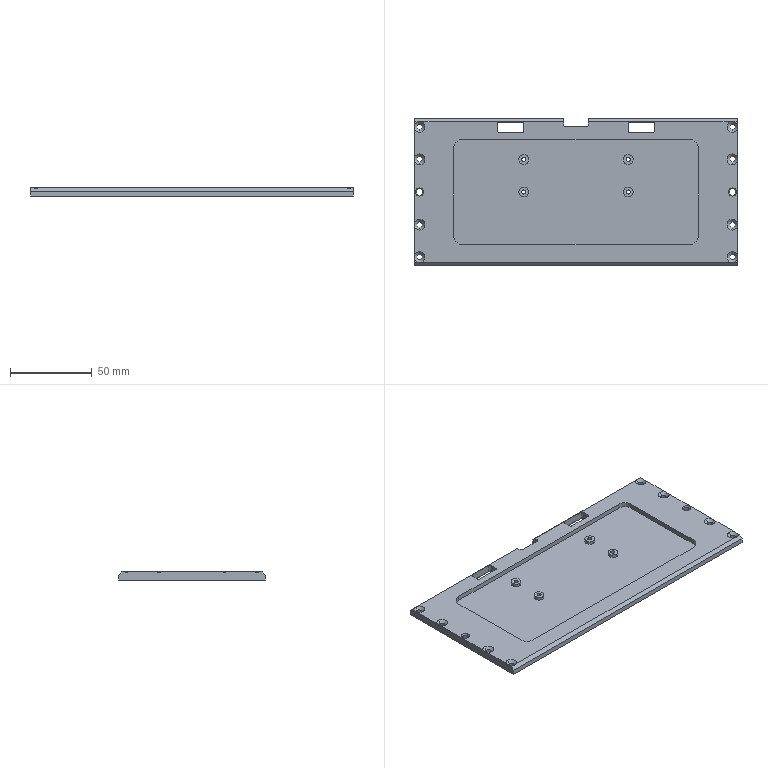NC program | NX | posted with a generic post | part box 198 x 90 x 5 mm
Lines 1737 to 2732 of 7766:
(ZLEVEL_PROFILE_COPY_1_COPY_COPY_COPY_COPY , TOOL : D2)
N3424 T17 M6
N3426 G54
N3428 G17 G0 G90 X-6.138 Y43.524 S9500 M3
N3430 G43 Z30. H17
N3432 Z-0.2
N3434 G94 G1 X-6.4 Y43.373 F1000.
N3436 G3 X-6.5 Y43.2 R0.2
N3438 G1 Y41. F1100.
N3440 X-3.016
N3442 G3 X-2.842 Y41.1 R0.2
N3444 G1 X-2.669 Y41.4
N3446 G0 X-6.138 Y43.724 Z-0.4
N3448 G1 X-6.4 Y43.573 F1000.
N3450 G3 X-6.5 Y43.4 R0.2
N3452 G1 Y41. F1100.
N3454 X-2.959
N3456 G3 X-2.786 Y41.1 R0.2
N3458 G1 X-2.613 Y41.4
N3460 G0 X-6.138 Y43.924 Z-0.6
N3462 G1 X-6.4 Y43.773 F1000.
N3464 G3 X-6.5 Y43.6 R0.2
N3466 G1 Y41. F1100.
N3468 X-2.895
N3470 G3 X-2.722 Y41.1 R0.2
N3472 G1 X-2.549 Y41.4
N3474 G0 X-6.138 Y44.124 Z-0.8
N3476 G1 X-6.4 Y43.973 F1000.
N3478 G3 X-6.5 Y43.8 R0.2
N3480 G1 Y41. F1100.
N3482 X-2.845
N3484 G3 X-2.672 Y41.1 R0.2
N3486 G1 X-2.499 Y41.4
N3488 G0 X-6.138 Y44.317 Z-1.
N3490 G1 X-6.4 Y44.166 F1000.
N3492 G3 X-6.5 Y43.993 R0.2
N3494 G1 Y41. F1100.
N3496 X-2.802
N3498 G3 X-2.629 Y41.1 R0.2
N3500 G1 X-2.456 Y41.4
N3502 G0 X-6.138 Y44.524 Z-1.2
N3504 G1 X-6.4 Y44.373 F1000.
N3506 G3 X-6.5 Y44.2 R0.2
N3508 G1 Y41. F1100.
N3510 X-2.761
N3512 G3 X-2.588 Y41.1 R0.2
N3514 G1 X-2.415 Y41.4
N3516 G0 X-6.138 Y44.724 Z-1.4
N3518 G1 X-6.4 Y44.573 F1000.
N3520 G3 X-6.5 Y44.4 R0.2
N3522 G1 Y41. F1100.
N3524 X-2.732
N3526 G3 X-2.559 Y41.1 R0.2
N3528 G1 X-2.386 Y41.4
N3530 G0 X-6.138 Y44.924 Z-1.6
N3532 G1 X-6.4 Y44.773 F1000.
N3534 G3 X-6.5 Y44.6 R0.2
N3536 G1 Y41. F1100.
N3538 X-2.716
N3540 G3 X-2.543 Y41.1 R0.2
N3542 G1 X-2.37 Y41.4
N3544 G0 X-6.132 Y45.097 Z-1.8
N3546 G1 X-6.4 Y44.943 F1000.
N3548 G3 X-6.5 Y44.769 R0.2
N3550 G1 Y41. F1100.
N3552 X-2.702
N3554 G3 X-2.529 Y41.1 R0.2
N3556 G1 X-2.355 Y41.4
N3558 G0 X-6.108 Y45.146 Z-2.
N3560 G1 X-6.4 Y44.977 F1000.
N3562 G3 X-6.5 Y44.804 R0.2
N3564 G1 Y41. F1100.
N3566 X-2.696
N3568 G3 X-2.522 Y41.1 R0.2
N3570 G1 X-2.349 Y41.4
N3572 G0 X-6.108 Y45.146 Z-2.2
N3574 G1 X-6.4 Y44.977 F1000.
N3576 G3 X-6.5 Y44.804 R0.2
N3578 G1 Y41. F1100.
N3580 X-2.696
N3582 G3 X-2.522 Y41.1 R0.2
N3584 G1 X-2.349 Y41.4
N3586 G0 X-6.108 Y45.146 Z-2.4
N3588 G1 X-6.4 Y44.977 F1000.
N3590 G3 X-6.5 Y44.804 R0.2
N3592 G1 Y41. F1100.
N3594 X-2.696
N3596 G3 X-2.522 Y41.1 R0.2
N3598 G1 X-2.349 Y41.4
N3600 G0 X-6.108 Y45.146 Z-2.6
N3602 G1 X-6.4 Y44.977 F1000.
N3604 G3 X-6.5 Y44.804 R0.2
N3606 G1 Y41. F1100.
N3608 X-2.696
N3610 G3 X-2.522 Y41.1 R0.2
N3612 G1 X-2.349 Y41.4
N3614 G0 X-6.108 Y45.146 Z-2.8
N3616 G1 X-6.4 Y44.977 F1000.
N3618 G3 X-6.5 Y44.804 R0.2
N3620 G1 Y41. F1100.
N3622 X-2.696
N3624 G3 X-2.522 Y41.1 R0.2
N3626 G1 X-2.349 Y41.4
N3628 G0 X-6.108 Y45.146 Z-3.
N3630 G1 X-6.4 Y44.977 F1000.
N3632 G3 X-6.5 Y44.804 R0.2
N3634 G1 Y41. F1100.
N3636 X-2.696
N3638 G3 X-2.522 Y41.1 R0.2
N3640 G1 X-2.349 Y41.4
N3642 G0 X-6.108 Y45.146 Z-3.2
N3644 G1 X-6.4 Y44.977 F1000.
N3646 G3 X-6.5 Y44.804 R0.2
N3648 G1 Y41. F1100.
N3650 X-2.696
N3652 G3 X-2.522 Y41.1 R0.2
N3654 G1 X-2.349 Y41.4
N3656 G0 X-6.108 Y45.146 Z-3.4
N3658 G1 X-6.4 Y44.977 F1000.
N3660 G3 X-6.5 Y44.804 R0.2
N3662 G1 Y41. F1100.
N3664 X-2.696
N3666 G3 X-2.522 Y41.1 R0.2
N3668 G1 X-2.349 Y41.4
N3670 G0 X-6.108 Y45.146 Z-3.6
N3672 G1 X-6.4 Y44.977 F1000.
N3674 G3 X-6.5 Y44.804 R0.2
N3676 G1 Y41. F1100.
N3678 X-2.696
N3680 G3 X-2.522 Y41.1 R0.2
N3682 G1 X-2.349 Y41.4
N3684 G0 X-6.108 Y45.146 Z-3.8
N3686 G1 X-6.4 Y44.977 F1000.
N3688 G3 X-6.5 Y44.804 R0.2
N3690 G1 Y41. F1100.
N3692 X-2.696
N3694 G3 X-2.522 Y41.1 R0.2
N3696 G1 X-2.349 Y41.4
N3698 G0 X-6.108 Y45.146 Z-4.
N3700 G1 X-6.4 Y44.977 F1000.
N3702 G3 X-6.5 Y44.804 R0.2
N3704 G1 Y41. F1100.
N3706 X-2.696
N3708 G3 X-2.522 Y41.1 R0.2
N3710 G1 X-2.349 Y41.4
N3712 G0 X-6.108 Y45.146 Z-4.2
N3714 G1 X-6.4 Y44.977 F1000.
N3716 G3 X-6.5 Y44.804 R0.2
N3718 G1 Y41. F1100.
N3720 X-2.696
N3722 G3 X-2.522 Y41.1 R0.2
N3724 G1 X-2.349 Y41.4
N3726 G0 X-6.108 Y45.146 Z-4.4
N3728 G1 X-6.4 Y44.977 F1000.
N3730 G3 X-6.5 Y44.804 R0.2
N3732 G1 Y41. F1100.
N3734 X-2.696
N3736 G3 X-2.522 Y41.1 R0.2
N3738 G1 X-2.349 Y41.4
N3740 G0 X-6.108 Y45.146 Z-4.6
N3742 G1 X-6.4 Y44.977 F1000.
N3744 G3 X-6.5 Y44.804 R0.2
N3746 G1 Y41. F1100.
N3748 X-2.696
N3750 G3 X-2.522 Y41.1 R0.2
N3752 G1 X-2.349 Y41.4
N3754 G0 X-6.108 Y45.146 Z-4.8
N3756 G1 X-6.4 Y44.977 F1000.
N3758 G3 X-6.5 Y44.804 R0.2
N3760 G1 Y41. F1100.
N3762 X-2.696
N3764 G3 X-2.522 Y41.1 R0.2
N3766 G1 X-2.349 Y41.4
N3768 G0 X-6.108 Y45.146 Z-5.
N3770 G1 X-6.4 Y44.977 F1000.
N3772 G3 X-6.5 Y44.804 R0.2
N3774 G1 Y41. F1100.
N3776 X-2.696
N3778 G3 X-2.522 Y41.1 R0.2
N3780 G1 X-2.349 Y41.4
N3782 G0 Z30.
N3784 X2.669
N3786 Z-0.2
N3788 G1 X2.842 Y41.1 F1000.
N3790 G3 X3.016 Y41. R0.2
N3792 G1 X6.5 F1100.
N3794 Y43.2
N3796 G3 X6.4 Y43.373 R0.2
N3798 G1 X6.138 Y43.524
N3800 G0 X2.613 Y41.4 Z-0.4
N3802 G1 X2.786 Y41.1 F1000.
N3804 G3 X2.959 Y41. R0.2
N3806 G1 X6.5 F1100.
N3808 Y43.4
N3810 G3 X6.4 Y43.573 R0.2
N3812 G1 X6.138 Y43.724
N3814 G0 X2.549 Y41.4 Z-0.6
N3816 G1 X2.722 Y41.1 F1000.
N3818 G3 X2.895 Y41. R0.2
N3820 G1 X6.5 F1100.
N3822 Y43.6
N3824 G3 X6.4 Y43.773 R0.2
N3826 G1 X6.138 Y43.924
N3828 G0 X2.499 Y41.4 Z-0.8
N3830 G1 X2.672 Y41.1 F1000.
N3832 G3 X2.845 Y41. R0.2
N3834 G1 X6.5 F1100.
N3836 Y43.8
N3838 G3 X6.4 Y43.973 R0.2
N3840 G1 X6.138 Y44.124
N3842 G0 X2.456 Y41.4 Z-1.
N3844 G1 X2.629 Y41.1 F1000.
N3846 G3 X2.802 Y41. R0.2
N3848 G1 X6.5 F1100.
N3850 Y43.993
N3852 G3 X6.4 Y44.166 R0.2
N3854 G1 X6.138 Y44.317
N3856 G0 X2.415 Y41.4 Z-1.2
N3858 G1 X2.588 Y41.1 F1000.
N3860 G3 X2.761 Y41. R0.2
N3862 G1 X6.5 F1100.
N3864 Y44.2
N3866 G3 X6.4 Y44.373 R0.2
N3868 G1 X6.138 Y44.524
N3870 G0 X2.386 Y41.4 Z-1.4
N3872 G1 X2.559 Y41.1 F1000.
N3874 G3 X2.732 Y41. R0.2
N3876 G1 X6.5 F1100.
N3878 Y44.4
N3880 G3 X6.4 Y44.573 R0.2
N3882 G1 X6.138 Y44.724
N3884 G0 X2.37 Y41.4 Z-1.6
N3886 G1 X2.543 Y41.1 F1000.
N3888 G3 X2.716 Y41. R0.2
N3890 G1 X6.5 F1100.
N3892 Y44.6
N3894 G3 X6.4 Y44.773 R0.2
N3896 G1 X6.138 Y44.924
N3898 G0 X2.355 Y41.4 Z-1.8
N3900 G1 X2.529 Y41.1 F1000.
N3902 G3 X2.702 Y41. R0.2
N3904 G1 X6.5 F1100.
N3906 Y44.769
N3908 G3 X6.4 Y44.943 R0.2
N3910 G1 X6.132 Y45.097
N3912 G0 X2.349 Y41.4 Z-2.
N3914 G1 X2.522 Y41.1 F1000.
N3916 G3 X2.696 Y41. R0.2
N3918 G1 X6.5 F1100.
N3920 Y44.804
N3922 G3 X6.4 Y44.977 R0.2
N3924 G1 X6.108 Y45.146
N3926 G0 X2.349 Y41.4 Z-2.2
N3928 G1 X2.522 Y41.1 F1000.
N3930 G3 X2.696 Y41. R0.2
N3932 G1 X6.5 F1100.
N3934 Y44.804
N3936 G3 X6.4 Y44.977 R0.2
N3938 G1 X6.108 Y45.146
N3940 G0 X2.349 Y41.4 Z-2.4
N3942 G1 X2.522 Y41.1 F1000.
N3944 G3 X2.696 Y41. R0.2
N3946 G1 X6.5 F1100.
N3948 Y44.804
N3950 G3 X6.4 Y44.977 R0.2
N3952 G1 X6.108 Y45.146
N3954 G0 X2.349 Y41.4 Z-2.6
N3956 G1 X2.522 Y41.1 F1000.
N3958 G3 X2.696 Y41. R0.2
N3960 G1 X6.5 F1100.
N3962 Y44.804
N3964 G3 X6.4 Y44.977 R0.2
N3966 G1 X6.108 Y45.146
N3968 G0 X2.349 Y41.4 Z-2.8
N3970 G1 X2.522 Y41.1 F1000.
N3972 G3 X2.696 Y41. R0.2
N3974 G1 X6.5 F1100.
N3976 Y44.804
N3978 G3 X6.4 Y44.977 R0.2
N3980 G1 X6.108 Y45.146
N3982 G0 X2.349 Y41.4 Z-3.
N3984 G1 X2.522 Y41.1 F1000.
N3986 G3 X2.696 Y41. R0.2
N3988 G1 X6.5 F1100.
N3990 Y44.804
N3992 G3 X6.4 Y44.977 R0.2
N3994 G1 X6.108 Y45.146
N3996 G0 X2.349 Y41.4 Z-3.2
N3998 G1 X2.522 Y41.1 F1000.
N4000 G3 X2.696 Y41. R0.2
N4002 G1 X6.5 F1100.
N4004 Y44.804
N4006 G3 X6.4 Y44.977 R0.2
N4008 G1 X6.108 Y45.146
N4010 G0 X2.349 Y41.4 Z-3.4
N4012 G1 X2.522 Y41.1 F1000.
N4014 G3 X2.696 Y41. R0.2
N4016 G1 X6.5 F1100.
N4018 Y44.804
N4020 G3 X6.4 Y44.977 R0.2
N4022 G1 X6.108 Y45.146
N4024 G0 X2.349 Y41.4 Z-3.6
N4026 G1 X2.522 Y41.1 F1000.
N4028 G3 X2.696 Y41. R0.2
N4030 G1 X6.5 F1100.
N4032 Y44.804
N4034 G3 X6.4 Y44.977 R0.2
N4036 G1 X6.108 Y45.146
N4038 G0 X2.349 Y41.4 Z-3.8
N4040 G1 X2.522 Y41.1 F1000.
N4042 G3 X2.696 Y41. R0.2
N4044 G1 X6.5 F1100.
N4046 Y44.804
N4048 G3 X6.4 Y44.977 R0.2
N4050 G1 X6.108 Y45.146
N4052 G0 X2.349 Y41.4 Z-4.
N4054 G1 X2.522 Y41.1 F1000.
N4056 G3 X2.696 Y41. R0.2
N4058 G1 X6.5 F1100.
N4060 Y44.804
N4062 G3 X6.4 Y44.977 R0.2
N4064 G1 X6.108 Y45.146
N4066 G0 X2.349 Y41.4 Z-4.2
N4068 G1 X2.522 Y41.1 F1000.
N4070 G3 X2.696 Y41. R0.2
N4072 G1 X6.5 F1100.
N4074 Y44.804
N4076 G3 X6.4 Y44.977 R0.2
N4078 G1 X6.108 Y45.146
N4080 G0 X2.349 Y41.4 Z-4.4
N4082 G1 X2.522 Y41.1 F1000.
N4084 G3 X2.696 Y41. R0.2
N4086 G1 X6.5 F1100.
N4088 Y44.804
N4090 G3 X6.4 Y44.977 R0.2
N4092 G1 X6.108 Y45.146
N4094 G0 X2.349 Y41.4 Z-4.6
N4096 G1 X2.522 Y41.1 F1000.
N4098 G3 X2.696 Y41. R0.2
N4100 G1 X6.5 F1100.
N4102 Y44.804
N4104 G3 X6.4 Y44.977 R0.2
N4106 G1 X6.108 Y45.146
N4108 G0 X2.349 Y41.4 Z-4.8
N4110 G1 X2.522 Y41.1 F1000.
N4112 G3 X2.696 Y41. R0.2
N4114 G1 X6.5 F1100.
N4116 Y44.804
N4118 G3 X6.4 Y44.977 R0.2
N4120 G1 X6.108 Y45.146
N4122 G0 X2.349 Y41.4 Z-5.
N4124 G1 X2.522 Y41.1 F1000.
N4126 G3 X2.696 Y41. R0.2
N4128 G1 X6.5 F1100.
N4130 Y44.804
N4132 G3 X6.4 Y44.977 R0.2
N4134 G1 X6.108 Y45.146
N4136 G0 Z30.
(ZLEVEL_PROFILE_COPY_1_COPY_COPY_COPY , TOOL : D2)
N4138 X-34.395 Y37.9
N4140 Z-0.2
N4142 G1 X-34.222 Y37.6 F1000.
N4144 G3 X-34.048 Y37.5 R0.2
N4146 G1 X-32.9 F1100.
N4148 Y37.653
N4150 Y38.648
N4152 G3 X-33. Y38.822 R0.2
N4154 G1 X-33.3 Y38.995
N4156 G0 X-34.395 Y37.9 Z-0.4
N4158 G1 X-34.222 Y37.6 F1000.
N4160 G3 X-34.048 Y37.5 R0.2
N4162 G1 X-32.9 F1100.
N4164 Y37.653
N4166 Y38.648
N4168 G3 X-33. Y38.822 R0.2
N4170 G1 X-33.3 Y38.995
N4172 G0 X-34.395 Y37.9 Z-0.6
N4174 G1 X-34.222 Y37.6 F1000.
N4176 G3 X-34.048 Y37.5 R0.2
N4178 G1 X-32.9 F1100.
N4180 Y37.653
N4182 Y38.648
N4184 G3 X-33. Y38.822 R0.2
N4186 G1 X-33.3 Y38.995
N4188 G0 X-34.395 Y37.9 Z-0.8
N4190 G1 X-34.222 Y37.6 F1000.
N4192 G3 X-34.048 Y37.5 R0.2
N4194 G1 X-32.9 F1100.
N4196 Y37.653
N4198 Y38.648
N4200 G3 X-33. Y38.822 R0.2
N4202 G1 X-33.3 Y38.995
N4204 G0 X-34.395 Y37.9 Z-1.
N4206 G1 X-34.222 Y37.6 F1000.
N4208 G3 X-34.048 Y37.5 R0.2
N4210 G1 X-32.9 F1100.
N4212 Y37.653
N4214 Y38.648
N4216 G3 X-33. Y38.822 R0.2
N4218 G1 X-33.3 Y38.995
N4220 G0 X-34.395 Y37.9 Z-1.2
N4222 G1 X-34.222 Y37.6 F1000.
N4224 G3 X-34.048 Y37.5 R0.2
N4226 G1 X-32.9 F1100.
N4228 Y37.653
N4230 Y38.648
N4232 G3 X-33. Y38.822 R0.2
N4234 G1 X-33.3 Y38.995
N4236 G0 X-34.395 Y37.9 Z-1.4
N4238 G1 X-34.222 Y37.6 F1000.
N4240 G3 X-34.048 Y37.5 R0.2
N4242 G1 X-32.9 F1100.
N4244 Y37.653
N4246 Y38.648
N4248 G3 X-33. Y38.822 R0.2
N4250 G1 X-33.3 Y38.995
N4252 G0 X-34.395 Y37.9 Z-1.6
N4254 G1 X-34.222 Y37.6 F1000.
N4256 G3 X-34.048 Y37.5 R0.2
N4258 G1 X-32.9 F1100.
N4260 Y37.653
N4262 Y38.648
N4264 G3 X-33. Y38.822 R0.2
N4266 G1 X-33.3 Y38.995
N4268 G0 X-34.395 Y37.9 Z-1.8
N4270 G1 X-34.222 Y37.6 F1000.
N4272 G3 X-34.048 Y37.5 R0.2
N4274 G1 X-32.9 F1100.
N4276 Y37.653
N4278 Y38.648
N4280 G3 X-33. Y38.822 R0.2
N4282 G1 X-33.3 Y38.995
N4284 G0 X-34.395 Y37.9 Z-2.
N4286 G1 X-34.222 Y37.6 F1000.
N4288 G3 X-34.048 Y37.5 R0.2
N4290 G1 X-32.9 F1100.
N4292 Y37.653
N4294 Y38.648
N4296 G3 X-33. Y38.822 R0.2
N4298 G1 X-33.3 Y38.995
N4300 G0 X-34.395 Y37.9 Z-2.2
N4302 G1 X-34.222 Y37.6 F1000.
N4304 G3 X-34.048 Y37.5 R0.2
N4306 G1 X-32.9 F1100.
N4308 Y37.653
N4310 Y38.648
N4312 G3 X-33. Y38.822 R0.2
N4314 G1 X-33.3 Y38.995
N4316 G0 X-34.395 Y37.9 Z-2.4
N4318 G1 X-34.222 Y37.6 F1000.
N4320 G3 X-34.048 Y37.5 R0.2
N4322 G1 X-32.9 F1100.
N4324 Y37.653
N4326 Y38.648
N4328 G3 X-33. Y38.822 R0.2
N4330 G1 X-33.3 Y38.995
N4332 G0 X-34.395 Y37.9 Z-2.6
N4334 G1 X-34.222 Y37.6 F1000.
N4336 G3 X-34.048 Y37.5 R0.2
N4338 G1 X-32.9 F1100.
N4340 Y37.653
N4342 Y38.648
N4344 G3 X-33. Y38.822 R0.2
N4346 G1 X-33.3 Y38.995
N4348 G0 X-34.395 Y37.9 Z-2.8
N4350 G1 X-34.222 Y37.6 F1000.
N4352 G3 X-34.048 Y37.5 R0.2
N4354 G1 X-32.9 F1100.
N4356 Y37.653
N4358 Y38.648
N4360 G3 X-33. Y38.822 R0.2
N4362 G1 X-33.3 Y38.995
N4364 G0 X-34.395 Y37.9 Z-3.
N4366 G1 X-34.222 Y37.6 F1000.
N4368 G3 X-34.048 Y37.5 R0.2
N4370 G1 X-32.9 F1100.
N4372 Y37.653
N4374 Y38.648
N4376 G3 X-33. Y38.822 R0.2
N4378 G1 X-33.3 Y38.995
N4380 G0 X-34.395 Y37.9 Z-3.2
N4382 G1 X-34.222 Y37.6 F1000.
N4384 G3 X-34.048 Y37.5 R0.2
N4386 G1 X-32.9 F1100.
N4388 Y37.653
N4390 Y38.648
N4392 G3 X-33. Y38.822 R0.2
N4394 G1 X-33.3 Y38.995
N4396 G0 X-34.395 Y37.9 Z-3.4
N4398 G1 X-34.222 Y37.6 F1000.
N4400 G3 X-34.048 Y37.5 R0.2
N4402 G1 X-32.9 F1100.
N4404 Y37.653
N4406 Y38.648
N4408 G3 X-33. Y38.822 R0.2
N4410 G1 X-33.3 Y38.995
N4412 G0 X-34.395 Y37.9 Z-3.6
N4414 G1 X-34.222 Y37.6 F1000.
N4416 G3 X-34.048 Y37.5 R0.2
N4418 G1 X-32.9 F1100.
N4420 Y37.653
N4422 Y38.648
N4424 G3 X-33. Y38.822 R0.2
N4426 G1 X-33.3 Y38.995
N4428 G0 X-34.395 Y37.9 Z-3.8
N4430 G1 X-34.222 Y37.6 F1000.
N4432 G3 X-34.048 Y37.5 R0.2
N4434 G1 X-32.9 F1100.
N4436 Y37.653
N4438 Y38.648
N4440 G3 X-33. Y38.822 R0.2
N4442 G1 X-33.3 Y38.995
N4444 G0 X-34.395 Y37.9 Z-4.
N4446 G1 X-34.222 Y37.6 F1000.
N4448 G3 X-34.048 Y37.5 R0.2
N4450 G1 X-32.9 F1100.
N4452 Y37.653
N4454 Y38.648
N4456 G3 X-33. Y38.822 R0.2
N4458 G1 X-33.3 Y38.995
N4460 G0 X-34.395 Y37.9 Z-4.2
N4462 G1 X-34.222 Y37.6 F1000.
N4464 G3 X-34.048 Y37.5 R0.2
N4466 G1 X-32.9 F1100.
N4468 Y37.653
N4470 Y38.648
N4472 G3 X-33. Y38.822 R0.2
N4474 G1 X-33.3 Y38.995
N4476 G0 X-34.395 Y37.9 Z-4.4
N4478 G1 X-34.222 Y37.6 F1000.
N4480 G3 X-34.048 Y37.5 R0.2
N4482 G1 X-32.9 F1100.
N4484 Y37.653
N4486 Y38.648
N4488 G3 X-33. Y38.822 R0.2
N4490 G1 X-33.3 Y38.995
N4492 G0 X-34.395 Y37.9 Z-4.6
N4494 G1 X-34.222 Y37.6 F1000.
N4496 G3 X-34.048 Y37.5 R0.2
N4498 G1 X-32.9 F1100.
N4500 Y37.653
N4502 Y38.648
N4504 G3 X-33. Y38.822 R0.2
N4506 G1 X-33.3 Y38.995
N4508 G0 X-34.395 Y37.9 Z-4.8
N4510 G1 X-34.222 Y37.6 F1000.
N4512 G3 X-34.048 Y37.5 R0.2
N4514 G1 X-32.9 F1100.
N4516 Y37.653
N4518 Y38.648
N4520 G3 X-33. Y38.822 R0.2
N4522 G1 X-33.3 Y38.995
N4524 G0 X-34.395 Y37.9 Z-5.
N4526 G1 X-34.222 Y37.6 F1000.
N4528 G3 X-34.048 Y37.5 R0.2
N4530 G1 X-32.9 F1100.
N4532 Y37.653
N4534 Y38.648
N4536 G3 X-33. Y38.822 R0.2
N4538 G1 X-33.3 Y38.995
N4540 G0 Z30.
N4542 Y40.205
N4544 Z-0.2
N4546 G1 X-33. Y40.378 F1000.
N4548 G3 X-32.9 Y40.552 R0.2
N4550 G1 Y41.7 F1100.
N4552 X-33.046
N4554 X-34.048
N4556 G3 X-34.222 Y41.6 R0.2
N4558 G1 X-34.395 Y41.3
N4560 G0 X-33.3 Y40.205 Z-0.4
N4562 G1 X-33. Y40.378 F1000.
N4564 G3 X-32.9 Y40.552 R0.2
N4566 G1 Y41.7 F1100.
N4568 X-33.046
N4570 X-34.048
N4572 G3 X-34.222 Y41.6 R0.2
N4574 G1 X-34.395 Y41.3
N4576 G0 X-33.3 Y40.205 Z-0.6
N4578 G1 X-33. Y40.378 F1000.
N4580 G3 X-32.9 Y40.552 R0.2
N4582 G1 Y41.7 F1100.
N4584 X-33.046
N4586 X-34.048
N4588 G3 X-34.222 Y41.6 R0.2
N4590 G1 X-34.395 Y41.3
N4592 G0 X-33.3 Y40.205 Z-0.8
N4594 G1 X-33. Y40.378 F1000.
N4596 G3 X-32.9 Y40.552 R0.2
N4598 G1 Y41.7 F1100.
N4600 X-33.046
N4602 X-34.048
N4604 G3 X-34.222 Y41.6 R0.2
N4606 G1 X-34.395 Y41.3
N4608 G0 X-33.3 Y40.205 Z-1.
N4610 G1 X-33. Y40.378 F1000.
N4612 G3 X-32.9 Y40.552 R0.2
N4614 G1 Y41.7 F1100.
N4616 X-33.046
N4618 X-34.048
N4620 G3 X-34.222 Y41.6 R0.2
N4622 G1 X-34.395 Y41.3
N4624 G0 X-33.3 Y40.205 Z-1.2
N4626 G1 X-33. Y40.378 F1000.
N4628 G3 X-32.9 Y40.552 R0.2
N4630 G1 Y41.7 F1100.
N4632 X-33.046
N4634 X-34.048
N4636 G3 X-34.222 Y41.6 R0.2
N4638 G1 X-34.395 Y41.3
N4640 G0 X-33.3 Y40.205 Z-1.4
N4642 G1 X-33. Y40.378 F1000.
N4644 G3 X-32.9 Y40.552 R0.2
N4646 G1 Y41.7 F1100.
N4648 X-33.046
N4650 X-34.048
N4652 G3 X-34.222 Y41.6 R0.2
N4654 G1 X-34.395 Y41.3
N4656 G0 X-33.3 Y40.205 Z-1.6
N4658 G1 X-33. Y40.378 F1000.
N4660 G3 X-32.9 Y40.552 R0.2
N4662 G1 Y41.7 F1100.
N4664 X-33.046
N4666 X-34.048
N4668 G3 X-34.222 Y41.6 R0.2
N4670 G1 X-34.395 Y41.3
N4672 G0 X-33.3 Y40.205 Z-1.8
N4674 G1 X-33. Y40.378 F1000.
N4676 G3 X-32.9 Y40.552 R0.2
N4678 G1 Y41.7 F1100.
N4680 X-33.046
N4682 X-34.048
N4684 G3 X-34.222 Y41.6 R0.2
N4686 G1 X-34.395 Y41.3
N4688 G0 X-33.3 Y40.205 Z-2.
N4690 G1 X-33. Y40.378 F1000.
N4692 G3 X-32.9 Y40.552 R0.2
N4694 G1 Y41.7 F1100.
N4696 X-33.046
N4698 X-34.048
N4700 G3 X-34.222 Y41.6 R0.2
N4702 G1 X-34.395 Y41.3
N4704 G0 X-33.3 Y40.205 Z-2.2
N4706 G1 X-33. Y40.378 F1000.
N4708 G3 X-32.9 Y40.552 R0.2
N4710 G1 Y41.7 F1100.
N4712 X-33.046
N4714 X-34.048
N4716 G3 X-34.222 Y41.6 R0.2
N4718 G1 X-34.395 Y41.3
N4720 G0 X-33.3 Y40.205 Z-2.4
N4722 G1 X-33. Y40.378 F1000.
N4724 G3 X-32.9 Y40.552 R0.2
N4726 G1 Y41.7 F1100.
N4728 X-33.046
N4730 X-34.048
N4732 G3 X-34.222 Y41.6 R0.2
N4734 G1 X-34.395 Y41.3
N4736 G0 X-33.3 Y40.205 Z-2.6
N4738 G1 X-33. Y40.378 F1000.
N4740 G3 X-32.9 Y40.552 R0.2
N4742 G1 Y41.7 F1100.
N4744 X-33.046
N4746 X-34.048
N4748 G3 X-34.222 Y41.6 R0.2
N4750 G1 X-34.395 Y41.3
N4752 G0 X-33.3 Y40.205 Z-2.8
N4754 G1 X-33. Y40.378 F1000.
N4756 G3 X-32.9 Y40.552 R0.2
N4758 G1 Y41.7 F1100.
N4760 X-33.046
N4762 X-34.048
N4764 G3 X-34.222 Y41.6 R0.2
N4766 G1 X-34.395 Y41.3
N4768 G0 X-33.3 Y40.205 Z-3.
N4770 G1 X-33. Y40.378 F1000.
N4772 G3 X-32.9 Y40.552 R0.2
N4774 G1 Y41.7 F1100.
N4776 X-33.046
N4778 X-34.048
N4780 G3 X-34.222 Y41.6 R0.2
N4782 G1 X-34.395 Y41.3
N4784 G0 X-33.3 Y40.205 Z-3.2
N4786 G1 X-33. Y40.378 F1000.
N4788 G3 X-32.9 Y40.552 R0.2
N4790 G1 Y41.7 F1100.
N4792 X-33.046
N4794 X-34.048
N4796 G3 X-34.222 Y41.6 R0.2
N4798 G1 X-34.395 Y41.3
N4800 G0 X-33.3 Y40.205 Z-3.4
N4802 G1 X-33. Y40.378 F1000.
N4804 G3 X-32.9 Y40.552 R0.2
N4806 G1 Y41.7 F1100.
N4808 X-33.046
N4810 X-34.048
N4812 G3 X-34.222 Y41.6 R0.2
N4814 G1 X-34.395 Y41.3
N4816 G0 X-33.3 Y40.205 Z-3.6
N4818 G1 X-33. Y40.378 F1000.
N4820 G3 X-32.9 Y40.552 R0.2
N4822 G1 Y41.7 F1100.
N4824 X-33.046
N4826 X-34.048
N4828 G3 X-34.222 Y41.6 R0.2
N4830 G1 X-34.395 Y41.3
N4832 G0 X-33.3 Y40.205 Z-3.8
N4834 G1 X-33. Y40.378 F1000.
N4836 G3 X-32.9 Y40.552 R0.2
N4838 G1 Y41.7 F1100.
N4840 X-33.046
N4842 X-34.048
N4844 G3 X-34.222 Y41.6 R0.2
N4846 G1 X-34.395 Y41.3
N4848 G0 X-33.3 Y40.205 Z-4.
N4850 G1 X-33. Y40.378 F1000.
N4852 G3 X-32.9 Y40.552 R0.2
N4854 G1 Y41.7 F1100.
N4856 X-33.003
N4858 X-34.048
N4860 G3 X-34.222 Y41.6 R0.2
N4862 G1 X-34.395 Y41.3
N4864 G0 X-33.3 Y40.205 Z-4.2
N4866 G1 X-33. Y40.378 F1000.
N4868 G3 X-32.9 Y40.552 R0.2
N4870 G1 Y41.7 F1100.
N4872 X-33.003
N4874 X-34.048
N4876 G3 X-34.222 Y41.6 R0.2
N4878 G1 X-34.395 Y41.3
N4880 G0 X-33.3 Y40.205 Z-4.4
N4882 G1 X-33. Y40.378 F1000.
N4884 G3 X-32.9 Y40.552 R0.2
N4886 G1 Y41.7 F1100.
N4888 X-33.003
N4890 X-34.048
N4892 G3 X-34.222 Y41.6 R0.2
N4894 G1 X-34.395 Y41.3
N4896 G0 X-33.3 Y40.206 Z-4.6
N4898 G1 X-33. Y40.379 F1000.
N4900 G3 X-32.9 Y40.552 R0.2
N4902 G1 Y41.7 F1100.
N4904 X-34.048
N4906 G3 X-34.221 Y41.6 R0.2
N4908 G1 X-34.394 Y41.3
N4910 G0 X-33.3 Y40.206 Z-4.8
N4912 G1 X-33. Y40.379 F1000.
N4914 G3 X-32.9 Y40.552 R0.2
N4916 G1 Y41.7 F1100.
N4918 X-34.048
N4920 G3 X-34.221 Y41.6 R0.2
N4922 G1 X-34.394 Y41.3
N4924 G0 X-33.3 Y40.206 Z-5.
N4926 G1 X-33. Y40.379 F1000.
N4928 G3 X-32.9 Y40.552 R0.2
N4930 G1 Y41.7 F1100.
N4932 X-34.048
N4934 G3 X-34.221 Y41.6 R0.2
N4936 G1 X-34.394 Y41.3
N4938 G0 Z30.
N4940 X-45.605
N4942 Z-0.2
N4944 G1 X-45.778 Y41.6 F1000.
N4946 G3 X-45.952 Y41.7 R0.2
N4948 G1 X-46.954 F1100.
N4950 X-47.1
N4952 Y40.552
N4954 G3 X-47. Y40.378 R0.2
N4956 G1 X-46.7 Y40.205
N4958 G0 X-45.605 Y41.3 Z-0.4
N4960 G1 X-45.778 Y41.6 F1000.
N4962 G3 X-45.952 Y41.7 R0.2
N4964 G1 X-46.954 F1100.
N4966 X-47.1
N4968 Y40.552
N4970 G3 X-47. Y40.378 R0.2
N4972 G1 X-46.7 Y40.205
N4974 G0 X-45.605 Y41.3 Z-0.6
N4976 G1 X-45.778 Y41.6 F1000.
N4978 G3 X-45.952 Y41.7 R0.2
N4980 G1 X-46.954 F1100.
N4982 X-47.1
N4984 Y40.552
N4986 G3 X-47. Y40.378 R0.2
N4988 G1 X-46.7 Y40.205
N4990 G0 X-45.605 Y41.3 Z-0.8
N4992 G1 X-45.778 Y41.6 F1000.
N4994 G3 X-45.952 Y41.7 R0.2
N4996 G1 X-46.954 F1100.
N4998 X-47.1
N5000 Y40.552
N5002 G3 X-47. Y40.378 R0.2
N5004 G1 X-46.7 Y40.205
N5006 G0 X-45.605 Y41.3 Z-1.
N5008 G1 X-45.778 Y41.6 F1000.
N5010 G3 X-45.952 Y41.7 R0.2
N5012 G1 X-46.954 F1100.
N5014 X-47.1
N5016 Y40.552
N5018 G3 X-47. Y40.378 R0.2
N5020 G1 X-46.7 Y40.205
N5022 G0 X-45.605 Y41.3 Z-1.2
N5024 G1 X-45.778 Y41.6 F1000.
N5026 G3 X-45.952 Y41.7 R0.2
N5028 G1 X-46.954 F1100.
N5030 X-47.1
N5032 Y40.552
N5034 G3 X-47. Y40.378 R0.2
N5036 G1 X-46.7 Y40.205
N5038 G0 X-45.605 Y41.3 Z-1.4
N5040 G1 X-45.778 Y41.6 F1000.
N5042 G3 X-45.952 Y41.7 R0.2
N5044 G1 X-46.954 F1100.
N5046 X-47.1
N5048 Y40.552
N5050 G3 X-47. Y40.378 R0.2
N5052 G1 X-46.7 Y40.205
N5054 G0 X-45.605 Y41.3 Z-1.6
N5056 G1 X-45.778 Y41.6 F1000.
N5058 G3 X-45.952 Y41.7 R0.2
N5060 G1 X-46.954 F1100.
N5062 X-47.1
N5064 Y40.552
N5066 G3 X-47. Y40.378 R0.2
N5068 G1 X-46.7 Y40.205
N5070 G0 X-45.605 Y41.3 Z-1.8
N5072 G1 X-45.778 Y41.6 F1000.
N5074 G3 X-45.952 Y41.7 R0.2
N5076 G1 X-46.954 F1100.
N5078 X-47.1
N5080 Y40.552
N5082 G3 X-47. Y40.378 R0.2
N5084 G1 X-46.7 Y40.205
N5086 G0 X-45.605 Y41.3 Z-2.
N5088 G1 X-45.778 Y41.6 F1000.
N5090 G3 X-45.952 Y41.7 R0.2
N5092 G1 X-46.954 F1100.
N5094 X-47.1
N5096 Y40.552
N5098 G3 X-47. Y40.378 R0.2
N5100 G1 X-46.7 Y40.205
N5102 G0 X-45.605 Y41.3 Z-2.2
N5104 G1 X-45.778 Y41.6 F1000.
N5106 G3 X-45.952 Y41.7 R0.2
N5108 G1 X-46.954 F1100.
N5110 X-47.1
N5112 Y40.552
N5114 G3 X-47. Y40.378 R0.2
N5116 G1 X-46.7 Y40.205
N5118 G0 X-45.605 Y41.3 Z-2.4
N5120 G1 X-45.778 Y41.6 F1000.
N5122 G3 X-45.952 Y41.7 R0.2
N5124 G1 X-46.954 F1100.
N5126 X-47.1
N5128 Y40.552
N5130 G3 X-47. Y40.378 R0.2
N5132 G1 X-46.7 Y40.205
N5134 G0 X-45.605 Y41.3 Z-2.6
N5136 G1 X-45.778 Y41.6 F1000.
N5138 G3 X-45.952 Y41.7 R0.2
N5140 G1 X-46.954 F1100.
N5142 X-47.1
N5144 Y40.552
N5146 G3 X-47. Y40.378 R0.2
N5148 G1 X-46.7 Y40.205
N5150 G0 X-45.605 Y41.3 Z-2.8
N5152 G1 X-45.778 Y41.6 F1000.
N5154 G3 X-45.952 Y41.7 R0.2
N5156 G1 X-46.954 F1100.
N5158 X-47.1
N5160 Y40.552
N5162 G3 X-47. Y40.378 R0.2
N5164 G1 X-46.7 Y40.205
N5166 G0 X-45.605 Y41.3 Z-3.
N5168 G1 X-45.778 Y41.6 F1000.
N5170 G3 X-45.952 Y41.7 R0.2
N5172 G1 X-46.954 F1100.
N5174 X-47.1
N5176 Y40.552
N5178 G3 X-47. Y40.378 R0.2
N5180 G1 X-46.7 Y40.205
N5182 G0 X-45.605 Y41.3 Z-3.2
N5184 G1 X-45.778 Y41.6 F1000.
N5186 G3 X-45.952 Y41.7 R0.2
N5188 G1 X-46.954 F1100.
N5190 X-47.1
N5192 Y40.552
N5194 G3 X-47. Y40.378 R0.2
N5196 G1 X-46.7 Y40.205
N5198 G0 X-45.605 Y41.3 Z-3.4
N5200 G1 X-45.778 Y41.6 F1000.
N5202 G3 X-45.952 Y41.7 R0.2
N5204 G1 X-46.954 F1100.
N5206 X-47.1
N5208 Y40.552
N5210 G3 X-47. Y40.378 R0.2
N5212 G1 X-46.7 Y40.205
N5214 G0 X-45.605 Y41.3 Z-3.6
N5216 G1 X-45.778 Y41.6 F1000.
N5218 G3 X-45.952 Y41.7 R0.2
N5220 G1 X-46.954 F1100.
N5222 X-47.1
N5224 Y40.552
N5226 G3 X-47. Y40.378 R0.2
N5228 G1 X-46.7 Y40.205
N5230 G0 X-45.605 Y41.3 Z-3.8
N5232 G1 X-45.778 Y41.6 F1000.
N5234 G3 X-45.952 Y41.7 R0.2
N5236 G1 X-46.954 F1100.
N5238 X-47.1
N5240 Y40.552
N5242 G3 X-47. Y40.378 R0.2
N5244 G1 X-46.7 Y40.205
N5246 G0 X-45.605 Y41.3 Z-4.
N5248 G1 X-45.778 Y41.6 F1000.
N5250 G3 X-45.952 Y41.7 R0.2
N5252 G1 X-46.997 F1100.
N5254 X-47.1
N5256 Y40.552
N5258 G3 X-47. Y40.378 R0.2
N5260 G1 X-46.7 Y40.205
N5262 G0 X-45.605 Y41.3 Z-4.2
N5264 G1 X-45.778 Y41.6 F1000.
N5266 G3 X-45.952 Y41.7 R0.2
N5268 G1 X-46.997 F1100.
N5270 X-47.1
N5272 Y40.552
N5274 G3 X-47. Y40.378 R0.2
N5276 G1 X-46.7 Y40.205
N5278 G0 X-45.605 Y41.3 Z-4.4
N5280 G1 X-45.778 Y41.6 F1000.
N5282 G3 X-45.952 Y41.7 R0.2
N5284 G1 X-46.997 F1100.
N5286 X-47.1
N5288 Y40.552
N5290 G3 X-47. Y40.378 R0.2
N5292 G1 X-46.7 Y40.205
N5294 G0 X-45.605 Y41.3 Z-4.6
N5296 G1 X-45.778 Y41.6 F1000.
N5298 G3 X-45.952 Y41.7 R0.2
N5300 G1 X-47.1 F1100.
N5302 Y40.552
N5304 G3 X-47. Y40.378 R0.2
N5306 G1 X-46.7 Y40.205
N5308 G0 X-45.605 Y41.3 Z-4.8
N5310 G1 X-45.778 Y41.6 F1000.
N5312 G3 X-45.952 Y41.7 R0.2
N5314 G1 X-47.1 F1100.
N5316 Y40.552
N5318 G3 X-47. Y40.378 R0.2
N5320 G1 X-46.7 Y40.205
N5322 G0 X-45.605 Y41.3 Z-5.
N5324 G1 X-45.778 Y41.6 F1000.
N5326 G3 X-45.952 Y41.7 R0.2
N5328 G1 X-47.1 F1100.
N5330 Y40.552
N5332 G3 X-47. Y40.378 R0.2
N5334 G1 X-46.7 Y40.205
N5336 G0 Z30.
N5338 Y38.995
N5340 Z-0.2
N5342 G1 X-47. Y38.822 F1000.
N5344 G3 X-47.1 Y38.648 R0.2
N5346 G1 Y37.653 F1100.
N5348 Y37.5
N5350 X-45.952
N5352 G3 X-45.778 Y37.6 R0.2
N5354 G1 X-45.605 Y37.9
N5356 G0 X-46.7 Y38.995 Z-0.4
N5358 G1 X-47. Y38.822 F1000.
N5360 G3 X-47.1 Y38.648 R0.2
N5362 G1 Y37.653 F1100.
N5364 Y37.5
N5366 X-45.952
N5368 G3 X-45.778 Y37.6 R0.2
N5370 G1 X-45.605 Y37.9
N5372 G0 X-46.7 Y38.995 Z-0.6
N5374 G1 X-47. Y38.822 F1000.
N5376 G3 X-47.1 Y38.648 R0.2
N5378 G1 Y37.653 F1100.
N5380 Y37.5
N5382 X-45.952
N5384 G3 X-45.778 Y37.6 R0.2
N5386 G1 X-45.605 Y37.9
N5388 G0 X-46.7 Y38.995 Z-0.8
N5390 G1 X-47. Y38.822 F1000.
N5392 G3 X-47.1 Y38.648 R0.2
N5394 G1 Y37.653 F1100.
N5396 Y37.5
N5398 X-45.952
N5400 G3 X-45.778 Y37.6 R0.2
N5402 G1 X-45.605 Y37.9